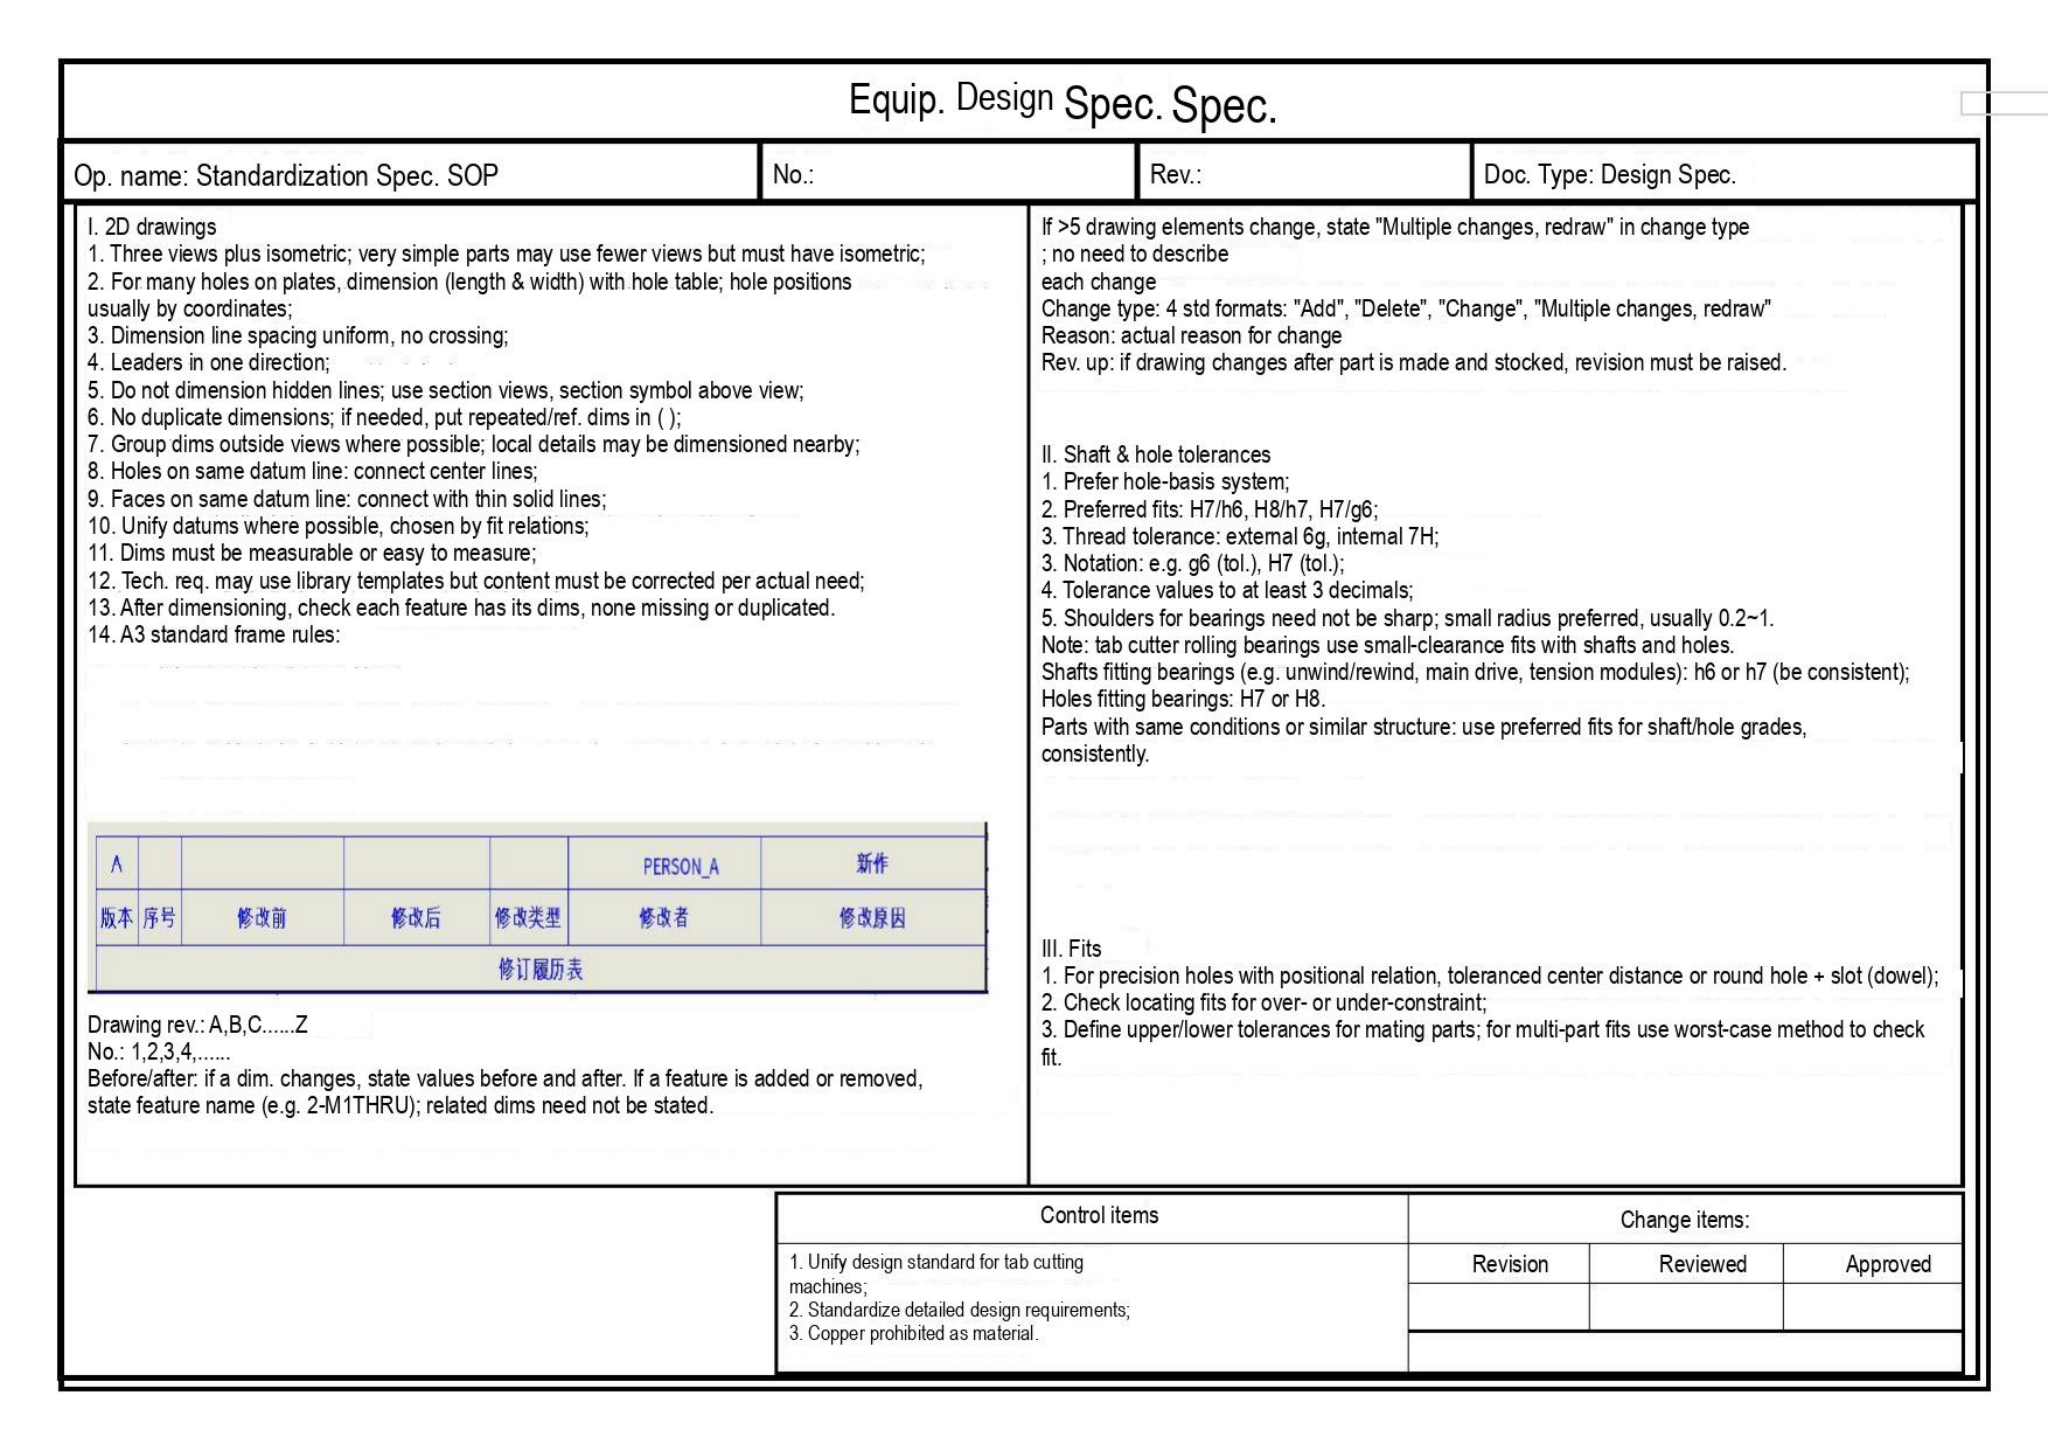Equip. Design Spec. Spec.

| Op. name: Standardization Spec. SOP | No.: | Rev.: | Doc. Type: Design Spec. |
|---|---|---|---|

I. 2D drawings
1. Three views plus isometric; very simple parts may use fewer views but must have isometric;
2. For many holes on plates, dimension (length & width) with hole table; hole positions usually by coordinates;
3. Dimension line spacing uniform, no crossing;
4. Leaders in one direction;
5. Do not dimension hidden lines; use section views, section symbol above view;
6. No duplicate dimensions; if needed, put repeated/ref. dims in ( );
7. Group dims outside views where possible; local details may be dimensioned nearby;
8. Holes on same datum line: connect center lines;
9. Faces on same datum line: connect with thin solid lines;
10. Unify datums where possible, chosen by fit relations;
11. Dims must be measurable or easy to measure;
12. Tech. req. may use library templates but content must be corrected per actual need;
13. After dimensioning, check each feature has its dims, none missing or duplicated.
14. A3 standard frame rules:

| A | | | | | PERSON_A | 新作 |
|---|---|---|---|---|---|---|
| 版本 | 序号 | 修改前 | 修改后 | 修改类型 | 修改者 | 修改原因 |
| 修订履历表 | | | | | | |

Drawing rev.: A,B,C......Z
No.: 1,2,3,4,......
Before/after: if a dim. changes, state values before and after. If a feature is added or removed, state feature name (e.g. 2-M1THRU); related dims need not be stated.

If >5 drawing elements change, state "Multiple changes, redraw" in change type
; no need to describe
each change
Change type: 4 std formats: "Add", "Delete", "Change", "Multiple changes, redraw"
Reason: actual reason for change
Rev. up: if drawing changes after part is made and stocked, revision must be raised.

II. Shaft & hole tolerances
1. Prefer hole-basis system;
2. Preferred fits: H7/h6, H8/h7, H7/g6;
3. Thread tolerance: external 6g, internal 7H;
3. Notation: e.g. g6 (tol.), H7 (tol.);
4. Tolerance values to at least 3 decimals;
5. Shoulders for bearings need not be sharp; small radius preferred, usually 0.2~1.
Note: tab cutter rolling bearings use small-clearance fits with shafts and holes.
Shafts fitting bearings (e.g. unwind/rewind, main drive, tension modules): h6 or h7 (be consistent);
Holes fitting bearings: H7 or H8.
Parts with same conditions or similar structure: use preferred fits for shaft/hole grades, consistently.

III. Fits
1. For precision holes with positional relation, toleranced center distance or round hole + slot (dowel);
2. Check locating fits for over- or under-constraint;
3. Define upper/lower tolerances for mating parts; for multi-part fits use worst-case method to check fit.

| Control items | Change items: | | |
|---|---|---|---|
| 1. Unify design standard for tab cutting machines;<br>2. Standardize detailed design requirements;<br>3. Copper prohibited as material. | Revision | Reviewed | Approved |
| | | | |
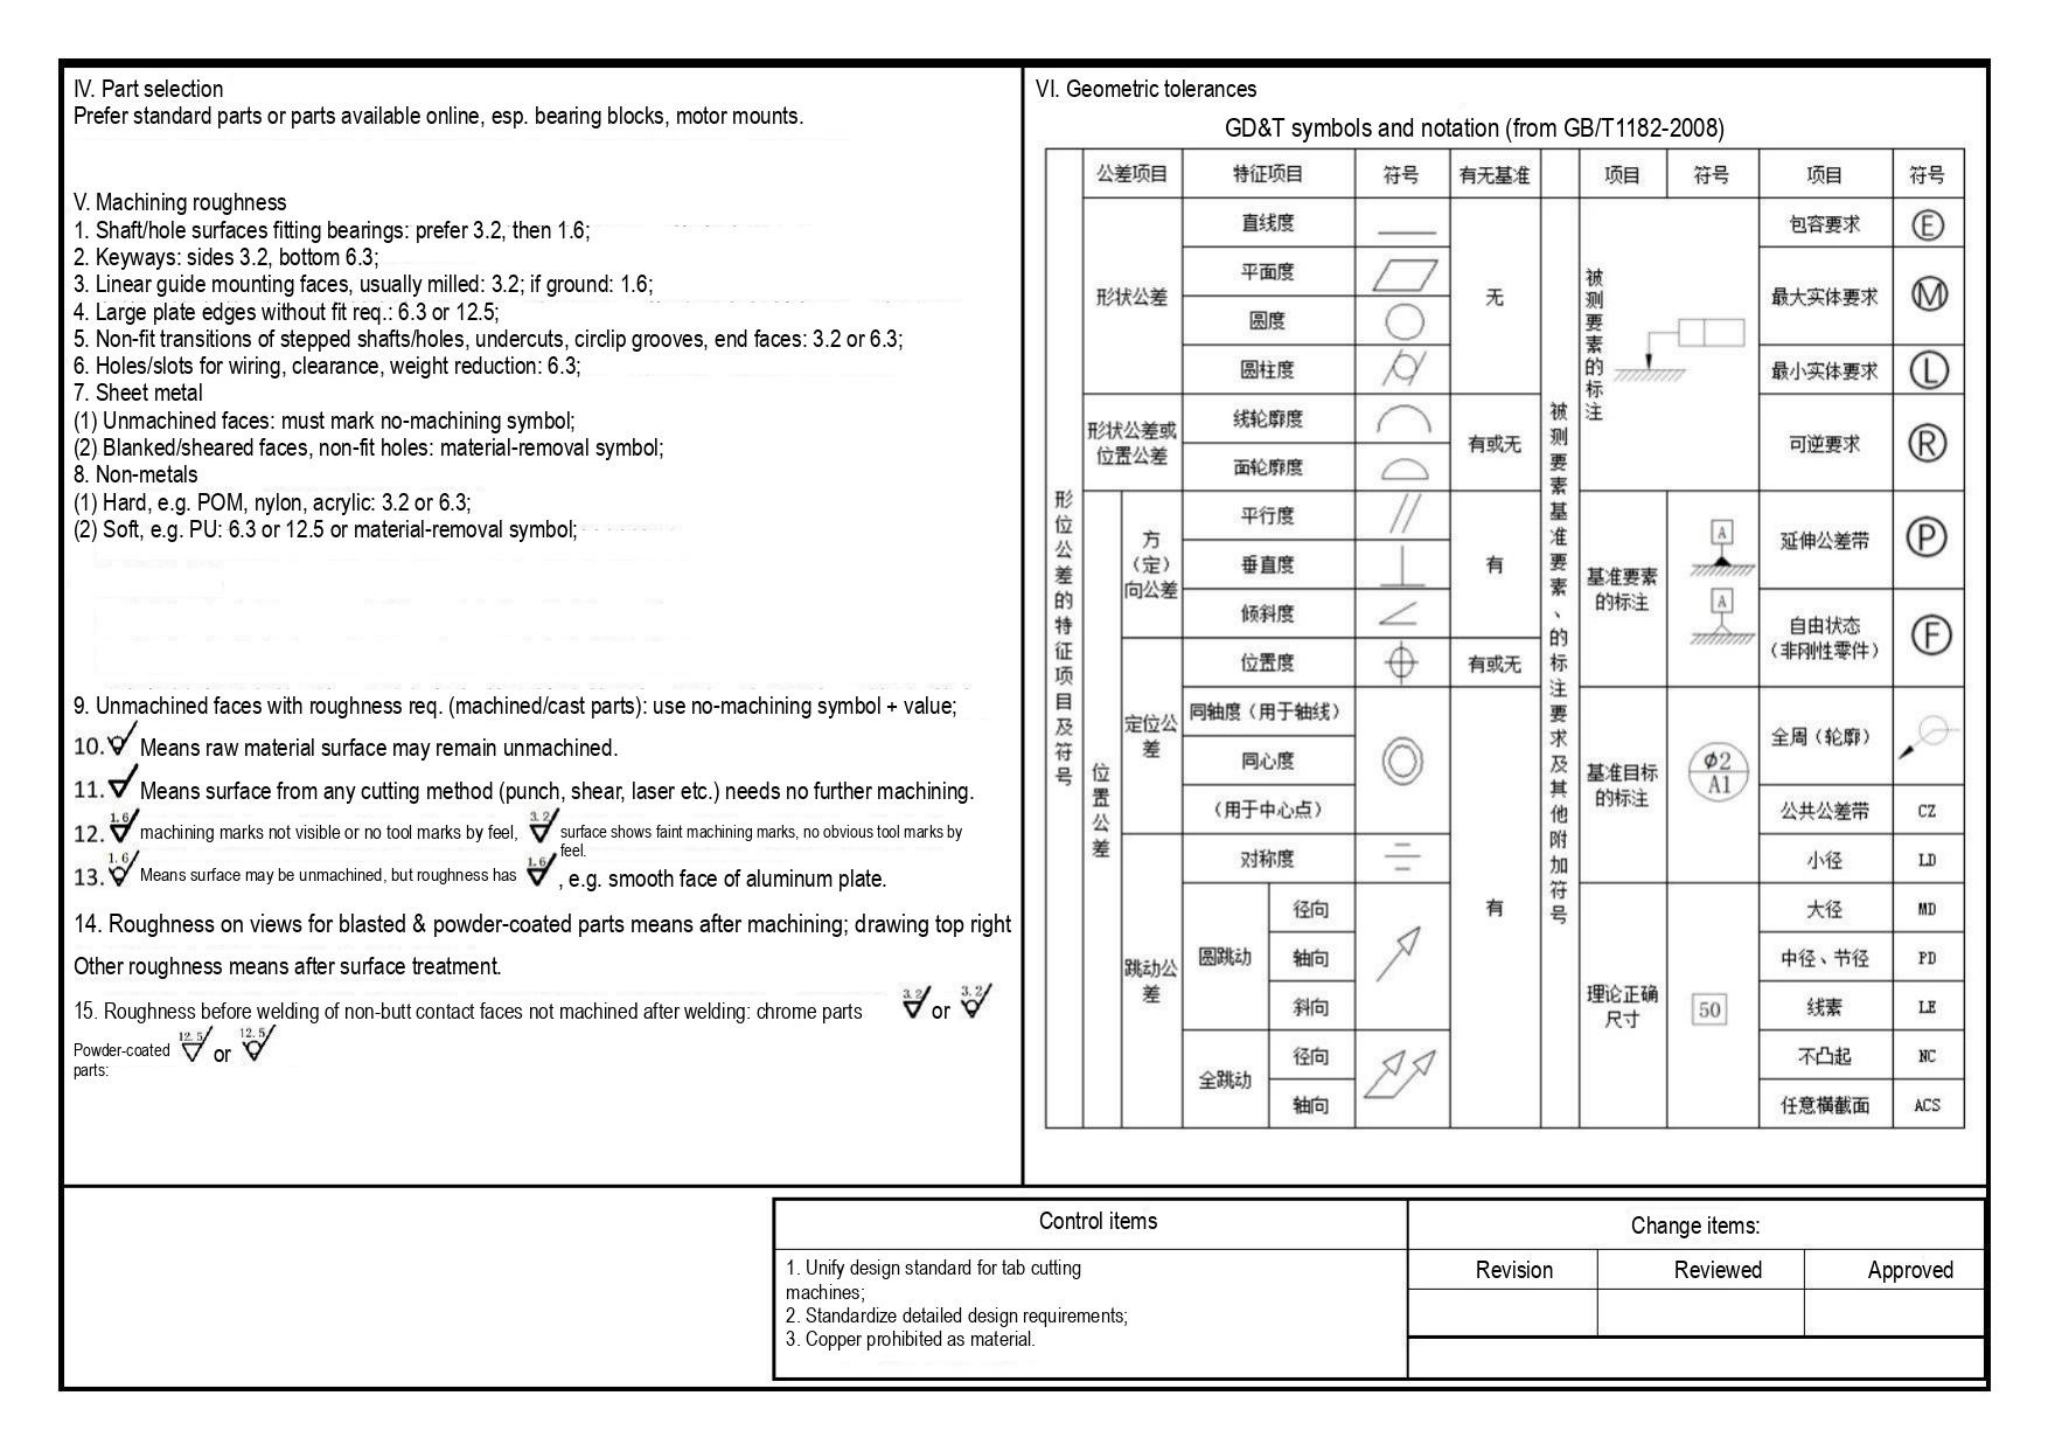IV. Part selection
Prefer standard parts or parts available online, esp. bearing blocks, motor mounts.

V. Machining roughness
1. Shaft/hole surfaces fitting bearings: prefer 3.2, then 1.6;
2. Keyways: sides 3.2, bottom 6.3;
3. Linear guide mounting faces, usually milled: 3.2; if ground: 1.6;
4. Large plate edges without fit req.: 6.3 or 12.5;
5. Non-fit transitions of stepped shafts/holes, undercuts, circlip grooves, end faces: 3.2 or 6.3;
6. Holes/slots for wiring, clearance, weight reduction: 6.3;
7. Sheet metal
(1) Unmachined faces: must mark no-machining symbol;
(2) Blanked/sheared faces, non-fit holes: material-removal symbol;
8. Non-metals
(1) Hard, e.g. POM, nylon, acrylic: 3.2 or 6.3;
(2) Soft, e.g. PU: 6.3 or 12.5 or material-removal symbol;

9. Unmachined faces with roughness req. (machined/cast parts): use no-machining symbol + value;
10. Means raw material surface may remain unmachined.
11. Means surface from any cutting method (punch, shear, laser etc.) needs no further machining.
12. 1.6 machining marks not visible or no tool marks by feel, 3.2 surface shows faint machining marks, no obvious tool marks by feel.
13. 1.6 Means surface may be unmachined, but roughness has 1.6, e.g. smooth face of aluminum plate.
14. Roughness on views for blasted & powder-coated parts means after machining; drawing top right
Other roughness means after surface treatment.
15. Roughness before welding of non-butt contact faces not machined after welding: chrome parts 3.2 or 3.2
Powder-coated parts: 12.5 or 12.5

VI. Geometric tolerances
GD&T symbols and notation (from GB/T1182-2008)

| | 公差项目 | | 特征项目 | | 符号 | 有无基准 | | 项目 | 符号 | 项目 | 符号 |
|---|---|---|---|---|---|---|---|---|---|---|---|
| 形位公差的特征项目及符号 | 形状公差 | | 直线度 | | | 无 | 被测要素基准要素、的标注要求及其他附加符号 | 被测要素的标注 | | 包容要求 | E |
| | | | 平面度 | | | | | | | 最大实体要求 | M |
| | | | 圆度 | | | | | | | | |
| | | | 圆柱度 | | | | | | | 最小实体要求 | L |
| | 形状公差或位置公差 | | 线轮廓度 | | | 有或无 | | | | 可逆要求 | R |
| | | | 面轮廓度 | | | | | | | | |
| | 位置公差 | 方（定）向公差 | 平行度 | | | 有 | | 基准要素的标注 | A | 延伸公差带 | P |
| | | | 垂直度 | | | | | | | | |
| | | | 倾斜度 | | | | | | A | 自由状态（非刚性零件） | F |
| | | 定位公差 | 位置度 | | | 有或无 | | | | | |
| | | | 同轴度（用于轴线） | | | 有 | | 基准目标的标注 | φ2 A1 | 全周（轮廓） | |
| | | | 同心度 | | | | | | | | |
| | | | （用于中心点） | | | | | | | 公共公差带 | CZ |
| | | | 对称度 | | | | | | | 小径 | LD |
| | | 跳动公差 | 圆跳动 | 径向 | | | | 理论正确尺寸 | 50 | 大径 | MD |
| | | | | 轴向 | | | | | | 中径、节径 | PD |
| | | | | 斜向 | | | | | | 线素 | LE |
| | | | 全跳动 | 径向 | | | | | | 不凸起 | NC |
| | | | | 轴向 | | | | | | 任意横截面 | ACS |

| Control items | Change items: | | |
|---|---|---|---|
| | Revision | Reviewed | Approved |
| 1. Unify design standard for tab cutting machines;<br>2. Standardize detailed design requirements;<br>3. Copper prohibited as material. | | | |
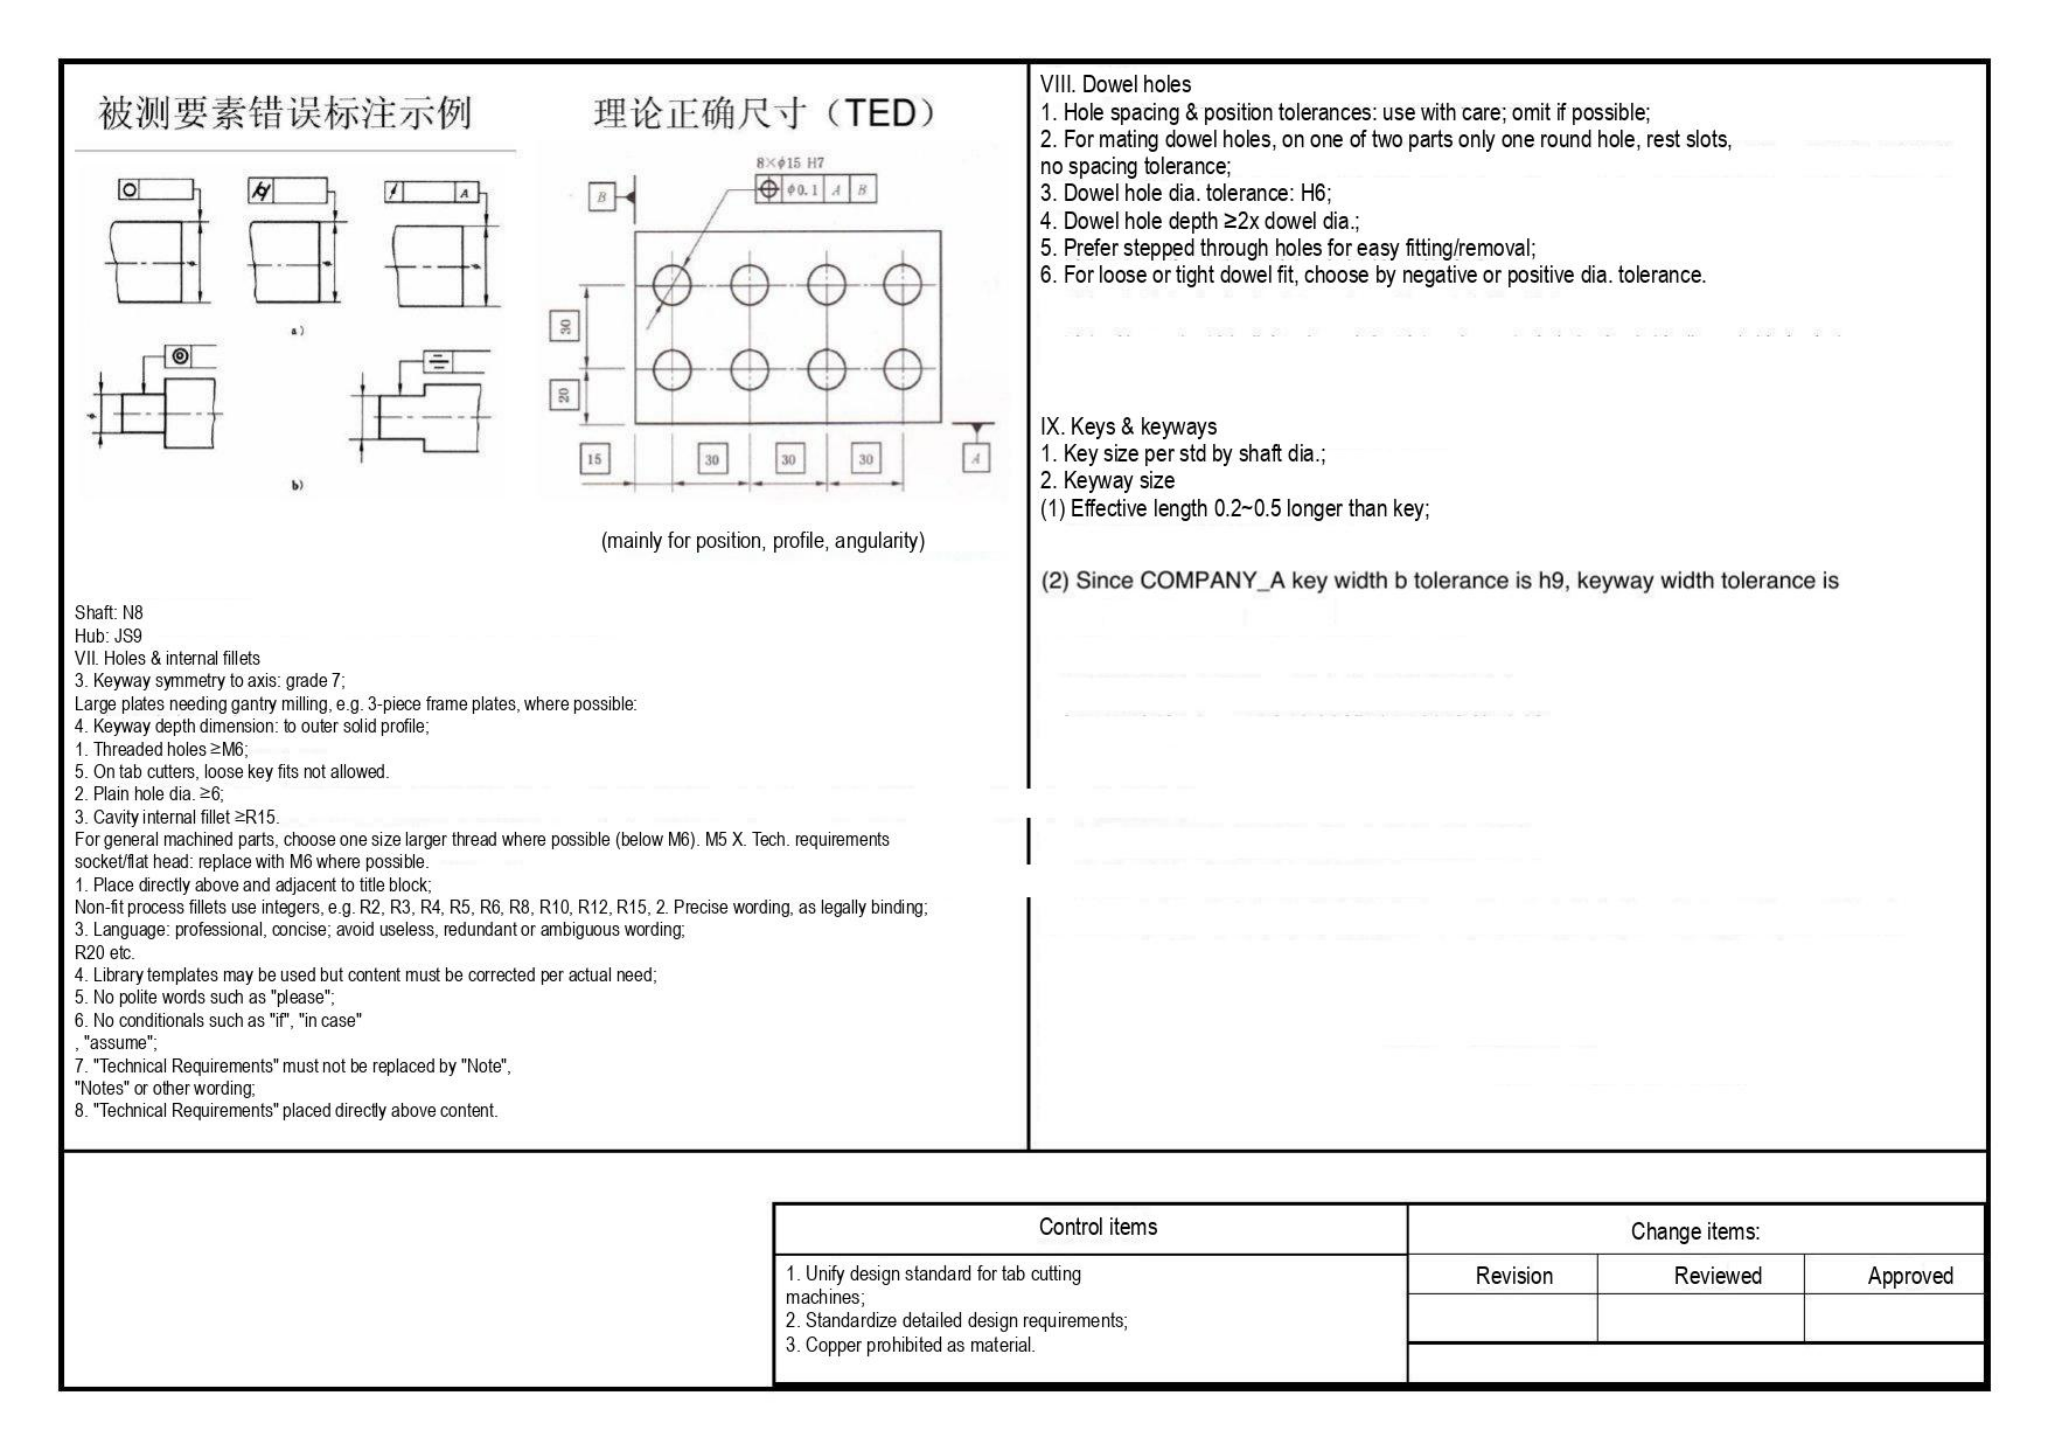被测要素错误标注示例

a)

b)

理论正确尺寸（TED）

8×ϕ15 H7

ϕ0.1 A B

B

30

20

15

30

30

30

A

(mainly for position, profile, angularity)

Shaft: N8
Hub: JS9
VII. Holes & internal fillets
3. Keyway symmetry to axis: grade 7;
Large plates needing gantry milling, e.g. 3-piece frame plates, where possible:
4. Keyway depth dimension: to outer solid profile;
1. Threaded holes ≥M6;
5. On tab cutters, loose key fits not allowed.
2. Plain hole dia. ≥6;
3. Cavity internal fillet ≥R15.
For general machined parts, choose one size larger thread where possible (below M6). M5 X. Tech. requirements
socket/flat head: replace with M6 where possible.
1. Place directly above and adjacent to title block;
Non-fit process fillets use integers, e.g. R2, R3, R4, R5, R6, R8, R10, R12, R15, 2. Precise wording, as legally binding;
3. Language: professional, concise; avoid useless, redundant or ambiguous wording;
R20 etc.
4. Library templates may be used but content must be corrected per actual need;
5. No polite words such as "please";
6. No conditionals such as "if", "in case"
, "assume";
7. "Technical Requirements" must not be replaced by "Note",
"Notes" or other wording;
8. "Technical Requirements" placed directly above content.

VIII. Dowel holes
1. Hole spacing & position tolerances: use with care; omit if possible;
2. For mating dowel holes, on one of two parts only one round hole, rest slots,
no spacing tolerance;
3. Dowel hole dia. tolerance: H6;
4. Dowel hole depth ≥2x dowel dia.;
5. Prefer stepped through holes for easy fitting/removal;
6. For loose or tight dowel fit, choose by negative or positive dia. tolerance.

IX. Keys & keyways
1. Key size per std by shaft dia.;
2. Keyway size
(1) Effective length 0.2~0.5 longer than key;

(2) Since COMPANY_A key width b tolerance is h9, keyway width tolerance is

| Control items | Change items: | | |
|---|---|---|---|
| | Revision | Reviewed | Approved |
| 1. Unify design standard for tab cutting machines;<br>2. Standardize detailed design requirements;<br>3. Copper prohibited as material. | | | |
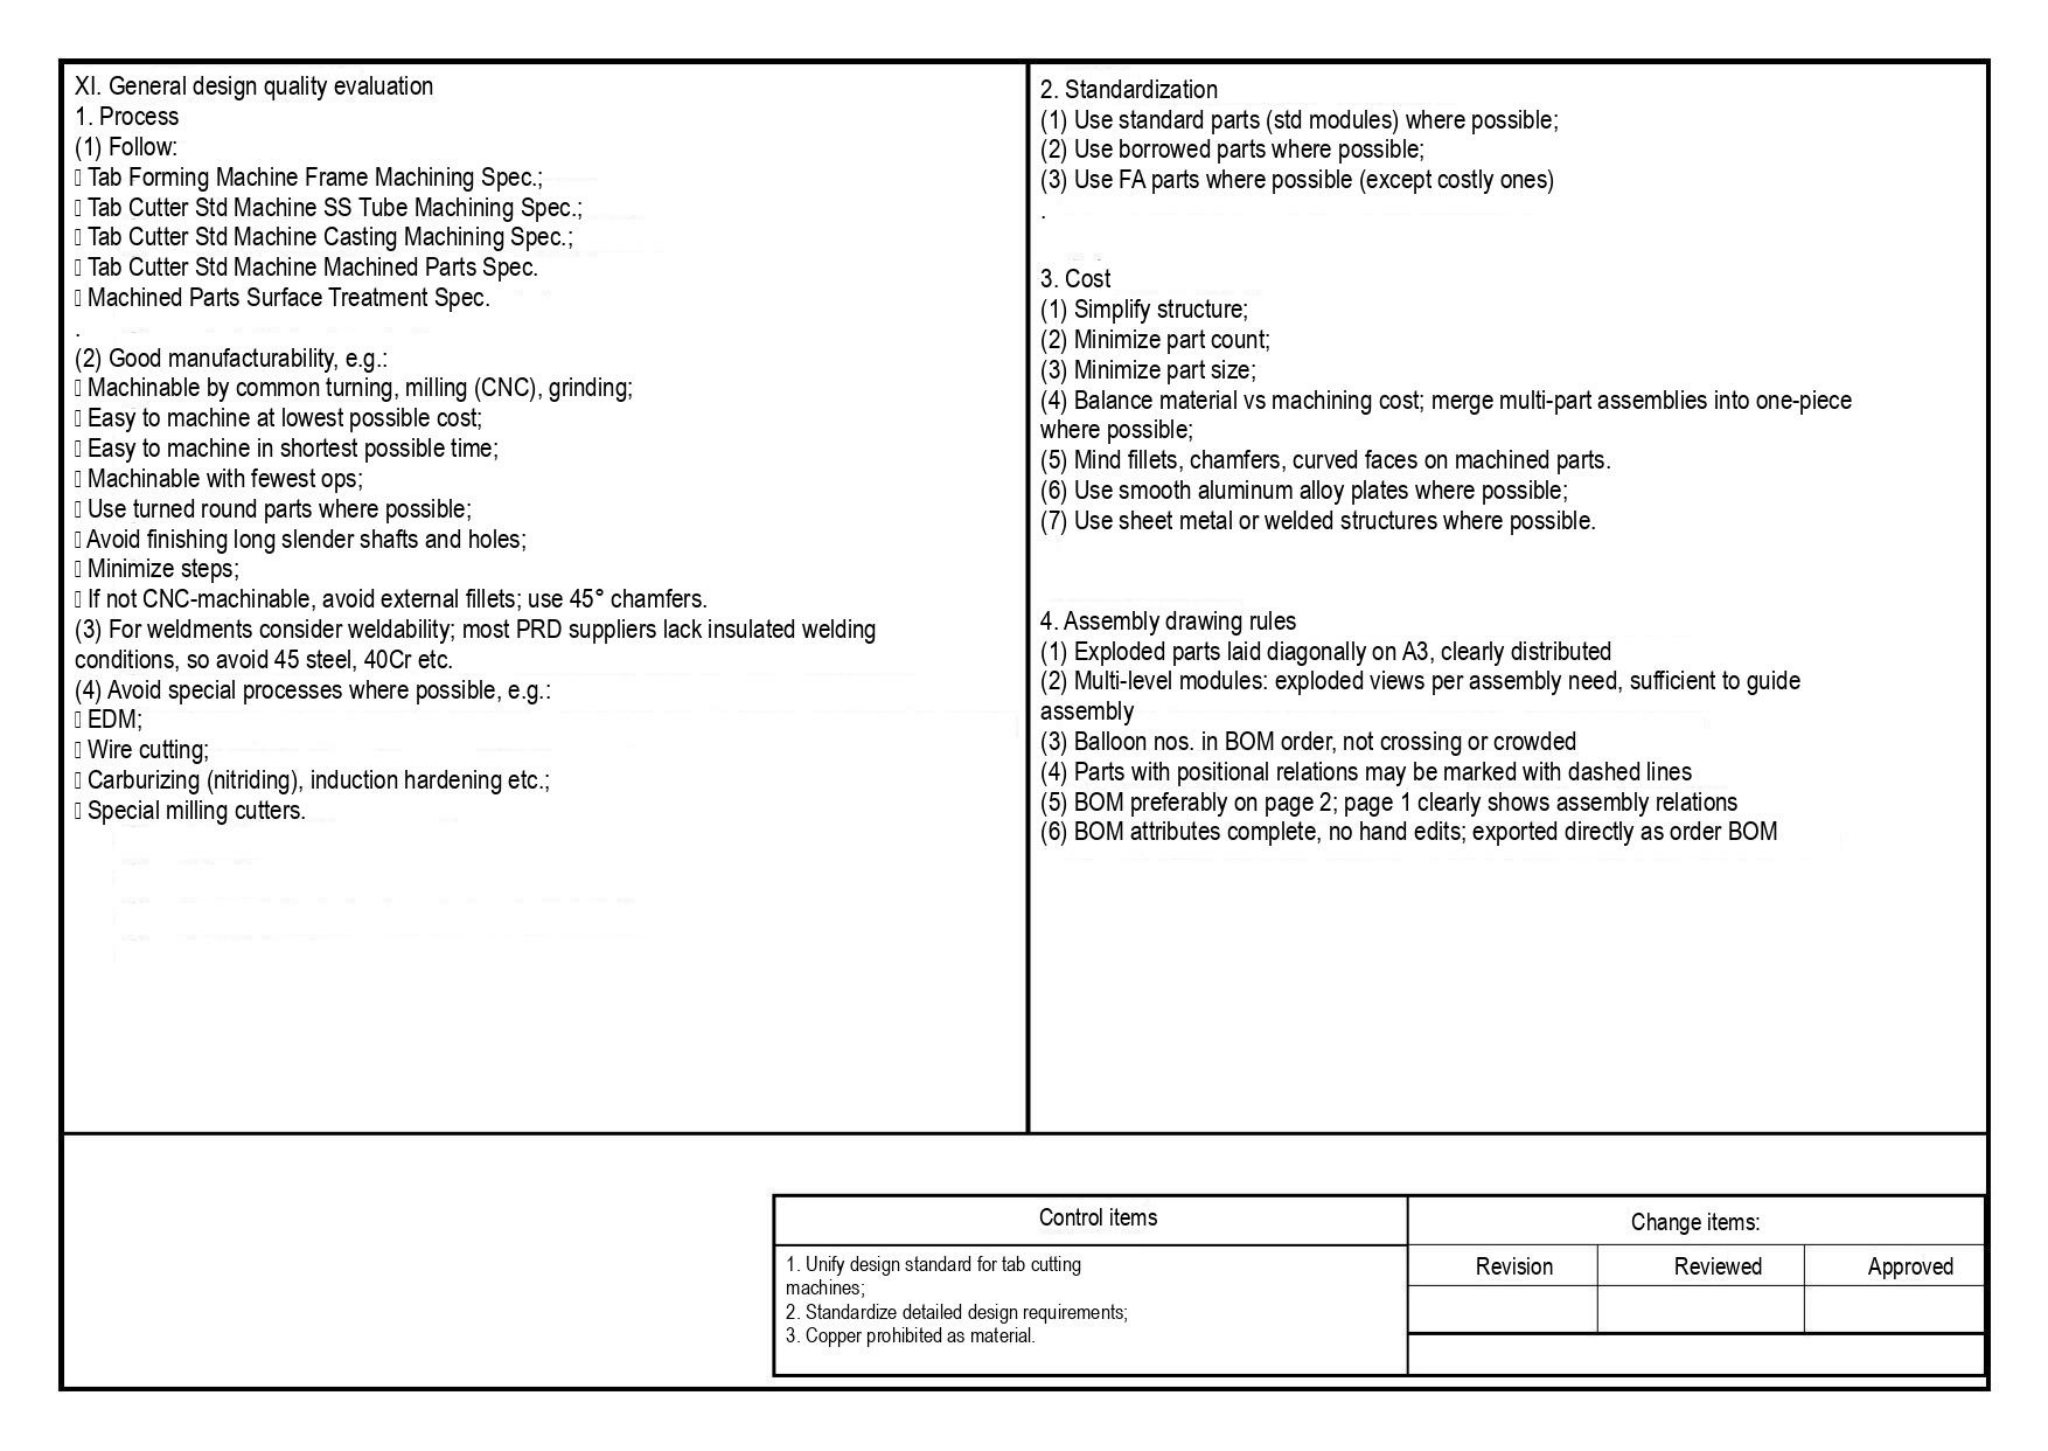XI. General design quality evaluation
1. Process
(1) Follow:
 Tab Forming Machine Frame Machining Spec.;
 Tab Cutter Std Machine SS Tube Machining Spec.;
 Tab Cutter Std Machine Casting Machining Spec.;
 Tab Cutter Std Machine Machined Parts Spec.
 Machined Parts Surface Treatment Spec.
.
(2) Good manufacturability, e.g.:
 Machinable by common turning, milling (CNC), grinding;
 Easy to machine at lowest possible cost;
 Easy to machine in shortest possible time;
 Machinable with fewest ops;
 Use turned round parts where possible;
 Avoid finishing long slender shafts and holes;
 Minimize steps;
 If not CNC-machinable, avoid external fillets; use 45° chamfers.
(3) For weldments consider weldability; most PRD suppliers lack insulated welding conditions, so avoid 45 steel, 40Cr etc.
(4) Avoid special processes where possible, e.g.:
 EDM;
 Wire cutting;
 Carburizing (nitriding), induction hardening etc.;
 Special milling cutters.

2. Standardization
(1) Use standard parts (std modules) where possible;
(2) Use borrowed parts where possible;
(3) Use FA parts where possible (except costly ones)
.

3. Cost
(1) Simplify structure;
(2) Minimize part count;
(3) Minimize part size;
(4) Balance material vs machining cost; merge multi-part assemblies into one-piece where possible;
(5) Mind fillets, chamfers, curved faces on machined parts.
(6) Use smooth aluminum alloy plates where possible;
(7) Use sheet metal or welded structures where possible.

4. Assembly drawing rules
(1) Exploded parts laid diagonally on A3, clearly distributed
(2) Multi-level modules: exploded views per assembly need, sufficient to guide assembly
(3) Balloon nos. in BOM order, not crossing or crowded
(4) Parts with positional relations may be marked with dashed lines
(5) BOM preferably on page 2; page 1 clearly shows assembly relations
(6) BOM attributes complete, no hand edits; exported directly as order BOM

| Control items | Change items: | | |
|---|---|---|---|
| 1. Unify design standard for tab cutting machines;<br>2. Standardize detailed design requirements;<br>3. Copper prohibited as material. | Revision | Reviewed | Approved |
| | | | |